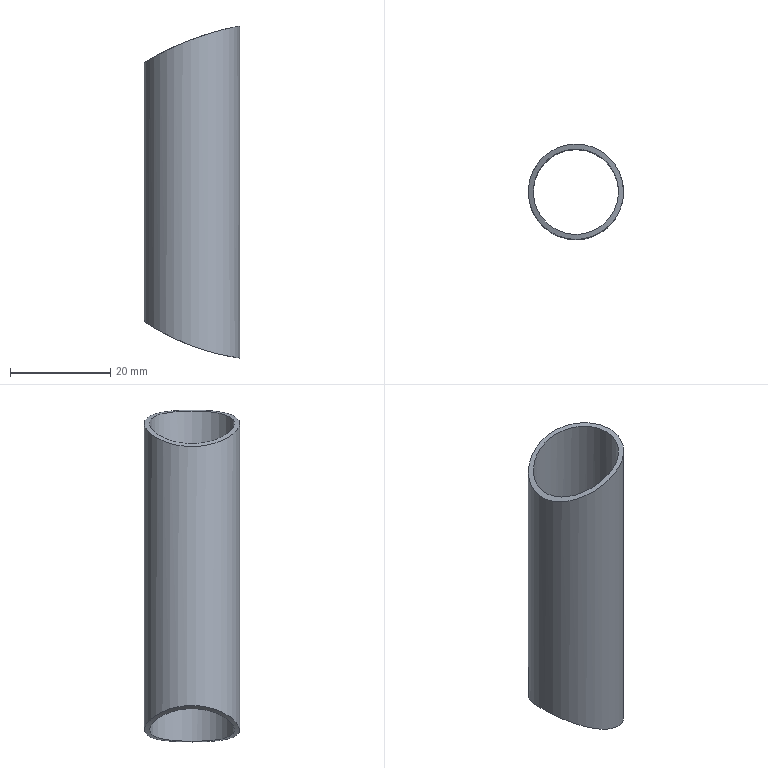Part | STEP file | 1-57.3 | 1 solid | 4 faces | box 19.001 x 19.001 x 66.2 mm | volume 3399 mm3 | cylinder 4 | commonest cylinder face diameters 17 x1 19 x1 92 x1 116.4 x1
STEP:
#1=CARTESIAN_POINT('',(0.,0.,0.));
#2=DIRECTION('',(0.,0.,1.));
#3=DIRECTION('',(1.,0.,0.));
#4=AXIS2_PLACEMENT_3D('',#1,#2,#3);
#5=CARTESIAN_POINT('',(9.5,0.00000001,33.1));
#6=VERTEX_POINT('',#5);
#7=CARTESIAN_POINT('',(9.5,0.000000021,33.1));
#8=CARTESIAN_POINT('',(9.5,1.036,33.1));
#9=CARTESIAN_POINT('',(8.992,4.143,33.002));
#10=CARTESIAN_POINT('',(7.036,6.692,32.594));
#11=CARTESIAN_POINT('',(3.324,9.242,31.592));
#12=CARTESIAN_POINT('',(0.8782,9.747,30.79));
#13=CARTESIAN_POINT('',(-3.995,8.997,28.801));
#14=CARTESIAN_POINT('',(-6.328,7.57,27.609));
#15=CARTESIAN_POINT('',(-9.203,3.377,26.002));
#16=CARTESIAN_POINT('',(-9.792,0.8976,25.625));
#17=CARTESIAN_POINT('',(-8.755,-5.155,26.247));
#18=CARTESIAN_POINT('',(-6.252,-7.864,27.729));
#19=CARTESIAN_POINT('',(-0.9257,-9.75,30.107));
#20=CARTESIAN_POINT('',(1.596,-9.694,31.037));
#21=CARTESIAN_POINT('',(6.765,-7.38,32.582));
#22=CARTESIAN_POINT('',(8.887,-4.697,32.98));
#23=CARTESIAN_POINT('',(9.438,-1.131,33.088));
#24=CARTESIAN_POINT('',(9.488,-0.6473,33.098));
#25=CARTESIAN_POINT('',(9.5,-0.1618,33.1));
#26=CARTESIAN_POINT('',(9.5,0.,33.1));
#27=B_SPLINE_CURVE_WITH_KNOTS('',3,(#7,#8,#9,#10,#11,#12,#13,#14,#15,#16,#17,#18,#19,#20,#21,#22,#23,#24,#25,#26),.UNSPECIFIED.,.F.,.F.,(4,1,2,2,2,2,2,2,2,1,4),(0.000000002,0.3333,1.,1.826,2.733,3.556,4.725,5.575,6.649,6.755,6.808),.UNSPECIFIED.);
#28=CARTESIAN_POINT('',(0.,0.,33.1));
#29=DIRECTION('',(0.,0.,-1.));
#30=DIRECTION('',(1.,0.,0.));
#31=AXIS2_PLACEMENT_3D('',#28,#29,#30);
#32=CYLINDRICAL_SURFACE('',#31,9.5);
#33=CARTESIAN_POINT('',(6.283,0.));
#34=CARTESIAN_POINT('',(6.233,0.00002118));
#35=CARTESIAN_POINT('',(6.131,0.0141));
#36=CARTESIAN_POINT('',(5.98,0.07863));
#37=CARTESIAN_POINT('',(5.83,0.1873));
#38=CARTESIAN_POINT('',(5.68,0.3429));
#39=CARTESIAN_POINT('',(5.531,0.5482));
#40=CARTESIAN_POINT('',(5.382,0.806));
#41=CARTESIAN_POINT('',(5.235,1.12));
#42=CARTESIAN_POINT('',(5.091,1.484));
#43=CARTESIAN_POINT('',(4.95,1.894));
#44=CARTESIAN_POINT('',(4.81,2.346));
#45=CARTESIAN_POINT('',(4.671,2.835));
#46=CARTESIAN_POINT('',(4.532,3.36));
#47=CARTESIAN_POINT('',(4.394,3.91));
#48=CARTESIAN_POINT('',(4.255,4.468));
#49=CARTESIAN_POINT('',(4.117,5.02));
#50=CARTESIAN_POINT('',(3.978,5.55));
#51=CARTESIAN_POINT('',(3.838,6.043));
#52=CARTESIAN_POINT('',(3.694,6.488));
#53=CARTESIAN_POINT('',(3.551,6.848));
#54=CARTESIAN_POINT('',(3.408,7.113));
#55=CARTESIAN_POINT('',(3.264,7.273));
#56=CARTESIAN_POINT('',(3.119,7.318));
#57=CARTESIAN_POINT('',(2.97,7.237));
#58=CARTESIAN_POINT('',(2.821,7.03));
#59=CARTESIAN_POINT('',(2.677,6.725));
#60=CARTESIAN_POINT('',(2.536,6.336));
#61=CARTESIAN_POINT('',(2.397,5.881));
#62=CARTESIAN_POINT('',(2.259,5.377));
#63=CARTESIAN_POINT('',(2.121,4.84));
#64=CARTESIAN_POINT('',(1.984,4.289));
#65=CARTESIAN_POINT('',(1.848,3.74));
#66=CARTESIAN_POINT('',(1.711,3.21));
#67=CARTESIAN_POINT('',(1.574,2.703));
#68=CARTESIAN_POINT('',(1.437,2.225));
#69=CARTESIAN_POINT('',(1.298,1.784));
#70=CARTESIAN_POINT('',(1.155,1.384));
#71=CARTESIAN_POINT('',(1.012,1.037));
#72=CARTESIAN_POINT('',(0.8697,0.7468));
#73=CARTESIAN_POINT('',(0.7278,0.508));
#74=CARTESIAN_POINT('',(0.5857,0.3183));
#75=CARTESIAN_POINT('',(0.4425,0.1747));
#76=CARTESIAN_POINT('',(0.2978,0.07458));
#77=CARTESIAN_POINT('',(0.1497,0.01389));
#78=CARTESIAN_POINT('',(0.04999,0.0002314));
#79=CARTESIAN_POINT('',(0.,0.));
#80=B_SPLINE_CURVE_WITH_KNOTS('',3,(#33,#34,#35,#36,#37,#38,#39,#40,#41,#42,#43,#44,#45,#46,#47,#48,#49,#50,#51,#52,#53,#54,#55,#56,#57,#58,#59,#60,#61,#62,#63,#64,#65,#66,#67,#68,#69,#70,#71,#72,#73,#74,#75,#76,#77,#78,#79),.UNSPECIFIED.,.F.,.F.,(4,1,1,1,1,1,1,1,1,1,1,1,1,1,1,1,1,1,1,1,1,1,1,1,1,1,1,1,1,1,1,1,1,1,1,1,1,1,1,1,1,1,1,1,4),(0.000000002,0.1547,0.3094,0.4641,0.6189,0.7736,0.9283,1.083,1.238,1.392,1.547,1.702,1.857,2.011,2.166,2.321,2.475,2.63,2.785,2.94,3.094,3.249,3.404,3.558,3.713,3.868,4.023,4.177,4.332,4.487,4.641,4.796,4.951,5.106,5.26,5.415,5.57,5.724,5.879,6.034,6.189,6.343,6.498,6.653,6.808),.QUASI_UNIFORM_KNOTS.);
#81=(GEOMETRIC_REPRESENTATION_CONTEXT(2)PARAMETRIC_REPRESENTATION_CONTEXT()REPRESENTATION_CONTEXT('',''));
#82=DEFINITIONAL_REPRESENTATION('',(#80),#81);
#83=PCURVE('',#32,#82);
#84=CARTESIAN_POINT('',(20.552,-33.1,-24.041));
#85=DIRECTION('',(0.,1.,0.));
#86=DIRECTION('',(-0.5164,0.,0.8564));
#87=AXIS2_PLACEMENT_3D('',#84,#85,#86);
#88=CYLINDRICAL_SURFACE('',#87,58.2);
#89=CARTESIAN_POINT('',(0.3515,33.1));
#90=CARTESIAN_POINT('',(0.3515,33.581));
#91=CARTESIAN_POINT('',(0.3503,34.542));
#92=CARTESIAN_POINT('',(0.3446,35.947));
#93=CARTESIAN_POINT('',(0.3353,37.277));
#94=CARTESIAN_POINT('',(0.3226,38.507));
#95=CARTESIAN_POINT('',(0.3068,39.613));
#96=CARTESIAN_POINT('',(0.2885,40.573));
#97=CARTESIAN_POINT('',(0.2678,41.361));
#98=CARTESIAN_POINT('',(0.2458,41.956));
#99=CARTESIAN_POINT('',(0.2226,42.364));
#100=CARTESIAN_POINT('',(0.1987,42.586));
#101=CARTESIAN_POINT('',(0.1745,42.623));
#102=CARTESIAN_POINT('',(0.1501,42.476));
#103=CARTESIAN_POINT('',(0.1262,42.15));
#104=CARTESIAN_POINT('',(0.1032,41.652));
#105=CARTESIAN_POINT('',(0.08148,40.991));
#106=CARTESIAN_POINT('',(0.06137,40.174));
#107=CARTESIAN_POINT('',(0.04331,39.211));
#108=CARTESIAN_POINT('',(0.02759,38.103));
#109=CARTESIAN_POINT('',(0.01512,36.896));
#110=CARTESIAN_POINT('',(0.006102,35.612));
#111=CARTESIAN_POINT('',(0.0007772,34.268));
#112=CARTESIAN_POINT('',(-0.0006513,32.886));
#113=CARTESIAN_POINT('',(0.002114,31.468));
#114=CARTESIAN_POINT('',(0.009037,30.094));
#115=CARTESIAN_POINT('',(0.01946,28.831));
#116=CARTESIAN_POINT('',(0.03303,27.675));
#117=CARTESIAN_POINT('',(0.04932,26.641));
#118=CARTESIAN_POINT('',(0.06791,25.739));
#119=CARTESIAN_POINT('',(0.08839,24.98));
#120=CARTESIAN_POINT('',(0.1104,24.374));
#121=CARTESIAN_POINT('',(0.1334,23.933));
#122=CARTESIAN_POINT('',(0.1571,23.664));
#123=CARTESIAN_POINT('',(0.181,23.569));
#124=CARTESIAN_POINT('',(0.205,23.654));
#125=CARTESIAN_POINT('',(0.2285,23.922));
#126=CARTESIAN_POINT('',(0.2515,24.378));
#127=CARTESIAN_POINT('',(0.2731,25.019));
#128=CARTESIAN_POINT('',(0.2925,25.817));
#129=CARTESIAN_POINT('',(0.3097,26.759));
#130=CARTESIAN_POINT('',(0.3242,27.831));
#131=CARTESIAN_POINT('',(0.336,29.018));
#132=CARTESIAN_POINT('',(0.3448,30.302));
#133=CARTESIAN_POINT('',(0.3503,31.678));
#134=CARTESIAN_POINT('',(0.3515,32.625));
#135=CARTESIAN_POINT('',(0.3515,33.1));
#136=B_SPLINE_CURVE_WITH_KNOTS('',3,(#89,#90,#91,#92,#93,#94,#95,#96,#97,#98,#99,#100,#101,#102,#103,#104,#105,#106,#107,#108,#109,#110,#111,#112,#113,#114,#115,#116,#117,#118,#119,#120,#121,#122,#123,#124,#125,#126,#127,#128,#129,#130,#131,#132,#133,#134,#135),.UNSPECIFIED.,.F.,.F.,(4,1,1,1,1,1,1,1,1,1,1,1,1,1,1,1,1,1,1,1,1,1,1,1,1,1,1,1,1,1,1,1,1,1,1,1,1,1,1,1,1,1,1,1,4),(0.000000002,0.1547,0.3094,0.4641,0.6189,0.7736,0.9283,1.083,1.238,1.392,1.547,1.702,1.857,2.011,2.166,2.321,2.475,2.63,2.785,2.94,3.094,3.249,3.404,3.558,3.713,3.868,4.023,4.177,4.332,4.487,4.641,4.796,4.951,5.106,5.26,5.415,5.57,5.724,5.879,6.034,6.189,6.343,6.498,6.653,6.808),.QUASI_UNIFORM_KNOTS.);
#137=(GEOMETRIC_REPRESENTATION_CONTEXT(2)PARAMETRIC_REPRESENTATION_CONTEXT()REPRESENTATION_CONTEXT('',''));
#138=DEFINITIONAL_REPRESENTATION('',(#136),#137);
#139=PCURVE('',#88,#138);
#140=SURFACE_CURVE('',#27,(#83,#139),.PCURVE_S1.);
#141=EDGE_CURVE('',#6,#6,#140,.T.);
#142=ORIENTED_EDGE('',*,*,#141,.F.);
#143=CARTESIAN_POINT('',(9.5,0.,-33.1));
#144=VERTEX_POINT('',#143);
#145=CARTESIAN_POINT('',(9.5,0.,33.1));
#146=DIRECTION('',(0.,0.,-1.));
#147=VECTOR('',#146,1.);
#148=LINE('',#145,#147);
#149=CARTESIAN_POINT('',(6.283,0.));
#150=DIRECTION('',(0.,1.));
#151=VECTOR('',#150,1.);
#152=LINE('',#149,#151);
#153=(GEOMETRIC_REPRESENTATION_CONTEXT(2)PARAMETRIC_REPRESENTATION_CONTEXT()REPRESENTATION_CONTEXT('',''));
#154=DEFINITIONAL_REPRESENTATION('',(#152),#153);
#155=PCURVE('',#32,#154);
#156=CARTESIAN_POINT('',(0.,0.));
#157=DIRECTION('',(0.,1.));
#158=VECTOR('',#157,1.);
#159=LINE('',#156,#158);
#160=(GEOMETRIC_REPRESENTATION_CONTEXT(2)PARAMETRIC_REPRESENTATION_CONTEXT()REPRESENTATION_CONTEXT('',''));
#161=DEFINITIONAL_REPRESENTATION('',(#159),#160);
#162=PCURVE('',#32,#161);
#163=SEAM_CURVE('',#148,(#155,#162),.PCURVE_S1.);
#164=EDGE_CURVE('',#6,#144,#163,.T.);
#165=ORIENTED_EDGE('',*,*,#164,.T.);
#166=CARTESIAN_POINT('',(9.5,0.,-33.1));
#167=CARTESIAN_POINT('',(9.5,-1.046,-33.1));
#168=CARTESIAN_POINT('',(8.981,-4.186,-33.025));
#169=CARTESIAN_POINT('',(6.985,-6.756,-32.698));
#170=CARTESIAN_POINT('',(3.23,-9.271,-31.791));
#171=CARTESIAN_POINT('',(0.8082,-9.745,-31.033));
#172=CARTESIAN_POINT('',(-3.78,-9.021,-29.136));
#173=CARTESIAN_POINT('',(-5.885,-7.822,-28.024));
#174=CARTESIAN_POINT('',(-8.869,-4.15,-26.254));
#175=CARTESIAN_POINT('',(-9.68,-1.751,-25.68));
#176=CARTESIAN_POINT('',(-9.166,4.378,-26.023));
#177=CARTESIAN_POINT('',(-6.919,7.261,-27.539));
#178=CARTESIAN_POINT('',(-2.119,9.491,-29.869));
#179=CARTESIAN_POINT('',(0.04298,9.745,-30.742));
#180=CARTESIAN_POINT('',(5.805,8.401,-32.573));
#181=CARTESIAN_POINT('',(8.729,5.438,-32.986));
#182=CARTESIAN_POINT('',(9.429,1.209,-33.09));
#183=CARTESIAN_POINT('',(9.486,0.6924,-33.098));
#184=CARTESIAN_POINT('',(9.5,0.1731,-33.1));
#185=CARTESIAN_POINT('',(9.5,0.,-33.1));
#186=B_SPLINE_CURVE_WITH_KNOTS('',3,(#166,#167,#168,#169,#170,#171,#172,#173,#174,#175,#176,#177,#178,#179,#180,#181,#182,#183,#184,#185),.UNSPECIFIED.,.T.,.F.,(1,3,1,2,2,2,2,2,2,2,1,3,1),(-0.05615,0.,0.3333,1.,1.807,2.617,3.432,4.581,5.323,6.601,6.713,6.769,7.103),.UNSPECIFIED.);
#187=CARTESIAN_POINT('',(0.,66.2));
#188=CARTESIAN_POINT('',(0.05086,66.2));
#189=CARTESIAN_POINT('',(0.1525,66.189));
#190=CARTESIAN_POINT('',(0.3046,66.14));
#191=CARTESIAN_POINT('',(0.4557,66.055));
#192=CARTESIAN_POINT('',(0.6064,65.929));
#193=CARTESIAN_POINT('',(0.7566,65.757));
#194=CARTESIAN_POINT('',(0.9062,65.532));
#195=CARTESIAN_POINT('',(1.055,65.248));
#196=CARTESIAN_POINT('',(1.2,64.908));
#197=CARTESIAN_POINT('',(1.343,64.516));
#198=CARTESIAN_POINT('',(1.483,64.074));
#199=CARTESIAN_POINT('',(1.623,63.586));
#200=CARTESIAN_POINT('',(1.763,63.053));
#201=CARTESIAN_POINT('',(1.902,62.487));
#202=CARTESIAN_POINT('',(2.04,61.907));
#203=CARTESIAN_POINT('',(2.178,61.328));
#204=CARTESIAN_POINT('',(2.317,60.767));
#205=CARTESIAN_POINT('',(2.457,60.237));
#206=CARTESIAN_POINT('',(2.599,59.766));
#207=CARTESIAN_POINT('',(2.741,59.379));
#208=CARTESIAN_POINT('',(2.884,59.092));
#209=CARTESIAN_POINT('',(3.029,58.92));
#210=CARTESIAN_POINT('',(3.177,58.879));
#211=CARTESIAN_POINT('',(3.33,58.989));
#212=CARTESIAN_POINT('',(3.475,59.226));
#213=CARTESIAN_POINT('',(3.618,59.57));
#214=CARTESIAN_POINT('',(3.758,60.001));
#215=CARTESIAN_POINT('',(3.897,60.498));
#216=CARTESIAN_POINT('',(4.035,61.041));
#217=CARTESIAN_POINT('',(4.172,61.609));
#218=CARTESIAN_POINT('',(4.308,62.182));
#219=CARTESIAN_POINT('',(4.444,62.742));
#220=CARTESIAN_POINT('',(4.58,63.282));
#221=CARTESIAN_POINT('',(4.717,63.791));
#222=CARTESIAN_POINT('',(4.856,64.262));
#223=CARTESIAN_POINT('',(4.999,64.688));
#224=CARTESIAN_POINT('',(5.14,65.049));
#225=CARTESIAN_POINT('',(5.279,65.351));
#226=CARTESIAN_POINT('',(5.419,65.6));
#227=CARTESIAN_POINT('',(5.559,65.799));
#228=CARTESIAN_POINT('',(5.699,65.953));
#229=CARTESIAN_POINT('',(5.841,66.067));
#230=CARTESIAN_POINT('',(5.985,66.144));
#231=CARTESIAN_POINT('',(6.133,66.19));
#232=CARTESIAN_POINT('',(6.233,66.2));
#233=CARTESIAN_POINT('',(6.283,66.2));
#234=B_SPLINE_CURVE_WITH_KNOTS('',3,(#187,#188,#189,#190,#191,#192,#193,#194,#195,#196,#197,#198,#199,#200,#201,#202,#203,#204,#205,#206,#207,#208,#209,#210,#211,#212,#213,#214,#215,#216,#217,#218,#219,#220,#221,#222,#223,#224,#225,#226,#227,#228,#229,#230,#231,#232,#233),.UNSPECIFIED.,.F.,.F.,(4,1,1,1,1,1,1,1,1,1,1,1,1,1,1,1,1,1,1,1,1,1,1,1,1,1,1,1,1,1,1,1,1,1,1,1,1,1,1,1,1,1,1,1,4),(0.,0.1538,0.3077,0.4615,0.6154,0.7692,0.9231,1.077,1.231,1.385,1.538,1.692,1.846,2.,2.154,2.308,2.462,2.615,2.769,2.923,3.077,3.231,3.385,3.538,3.692,3.846,4.,4.154,4.308,4.462,4.615,4.769,4.923,5.077,5.231,5.385,5.538,5.692,5.846,6.,6.154,6.308,6.461,6.615,6.769),.QUASI_UNIFORM_KNOTS.);
#235=(GEOMETRIC_REPRESENTATION_CONTEXT(2)PARAMETRIC_REPRESENTATION_CONTEXT()REPRESENTATION_CONTEXT('',''));
#236=DEFINITIONAL_REPRESENTATION('',(#234),#235);
#237=PCURVE('',#32,#236);
#238=CARTESIAN_POINT('',(16.089,-33.1,12.426));
#239=DIRECTION('',(0.,1.,0.));
#240=DIRECTION('',(-0.1432,0.,-0.9897));
#241=AXIS2_PLACEMENT_3D('',#238,#239,#240);
#242=CYLINDRICAL_SURFACE('',#241,46.);
#243=CARTESIAN_POINT('',(0.,33.1));
#244=CARTESIAN_POINT('',(-0.000003529,32.617));
#245=CARTESIAN_POINT('',(0.00162,31.651));
#246=CARTESIAN_POINT('',(0.00879,30.239));
#247=CARTESIAN_POINT('',(0.02063,28.903));
#248=CARTESIAN_POINT('',(0.03674,27.668));
#249=CARTESIAN_POINT('',(0.05668,26.557));
#250=CARTESIAN_POINT('',(0.08002,25.594));
#251=CARTESIAN_POINT('',(0.1064,24.804));
#252=CARTESIAN_POINT('',(0.1345,24.213));
#253=CARTESIAN_POINT('',(0.164,23.814));
#254=CARTESIAN_POINT('',(0.1943,23.604));
#255=CARTESIAN_POINT('',(0.2252,23.582));
#256=CARTESIAN_POINT('',(0.2561,23.745));
#257=CARTESIAN_POINT('',(0.2864,24.087));
#258=CARTESIAN_POINT('',(0.3156,24.599));
#259=CARTESIAN_POINT('',(0.3433,25.274));
#260=CARTESIAN_POINT('',(0.3688,26.101));
#261=CARTESIAN_POINT('',(0.3918,27.076));
#262=CARTESIAN_POINT('',(0.4116,28.179));
#263=CARTESIAN_POINT('',(0.4273,29.382));
#264=CARTESIAN_POINT('',(0.4388,30.671));
#265=CARTESIAN_POINT('',(0.4455,32.029));
#266=CARTESIAN_POINT('',(0.447,33.442));
#267=CARTESIAN_POINT('',(0.4427,34.884));
#268=CARTESIAN_POINT('',(0.4334,36.223));
#269=CARTESIAN_POINT('',(0.4195,37.472));
#270=CARTESIAN_POINT('',(0.4017,38.612));
#271=CARTESIAN_POINT('',(0.3805,39.633));
#272=CARTESIAN_POINT('',(0.3565,40.522));
#273=CARTESIAN_POINT('',(0.3302,41.269));
#274=CARTESIAN_POINT('',(0.3022,41.859));
#275=CARTESIAN_POINT('',(0.273,42.287));
#276=CARTESIAN_POINT('',(0.2429,42.547));
#277=CARTESIAN_POINT('',(0.2125,42.631));
#278=CARTESIAN_POINT('',(0.182,42.533));
#279=CARTESIAN_POINT('',(0.1517,42.244));
#280=CARTESIAN_POINT('',(0.1233,41.774));
#281=CARTESIAN_POINT('',(0.09705,41.139));
#282=CARTESIAN_POINT('',(0.07321,40.35));
#283=CARTESIAN_POINT('',(0.05211,39.419));
#284=CARTESIAN_POINT('',(0.03407,38.359));
#285=CARTESIAN_POINT('',(0.01942,37.183));
#286=CARTESIAN_POINT('',(0.008493,35.904));
#287=CARTESIAN_POINT('',(0.001587,34.525));
#288=CARTESIAN_POINT('',(-0.00001821,33.576));
#289=CARTESIAN_POINT('',(0.,33.1));
#290=B_SPLINE_CURVE_WITH_KNOTS('',3,(#243,#244,#245,#246,#247,#248,#249,#250,#251,#252,#253,#254,#255,#256,#257,#258,#259,#260,#261,#262,#263,#264,#265,#266,#267,#268,#269,#270,#271,#272,#273,#274,#275,#276,#277,#278,#279,#280,#281,#282,#283,#284,#285,#286,#287,#288,#289),.UNSPECIFIED.,.T.,.F.,(4,1,1,1,1,1,1,1,1,1,1,1,1,1,1,1,1,1,1,1,1,1,1,1,1,1,1,1,1,1,1,1,1,1,1,1,1,1,1,1,1,1,1,1,4),(0.,0.1538,0.3077,0.4615,0.6154,0.7692,0.9231,1.077,1.231,1.385,1.538,1.692,1.846,2.,2.154,2.308,2.462,2.615,2.769,2.923,3.077,3.231,3.385,3.538,3.692,3.846,4.,4.154,4.308,4.462,4.615,4.769,4.923,5.077,5.231,5.385,5.538,5.692,5.846,6.,6.154,6.308,6.461,6.615,6.769),.QUASI_UNIFORM_KNOTS.);
#291=(GEOMETRIC_REPRESENTATION_CONTEXT(2)PARAMETRIC_REPRESENTATION_CONTEXT()REPRESENTATION_CONTEXT('',''));
#292=DEFINITIONAL_REPRESENTATION('',(#290),#291);
#293=PCURVE('',#242,#292);
#294=SURFACE_CURVE('',#186,(#237,#293),.PCURVE_S1.);
#295=EDGE_CURVE('',#144,#144,#294,.T.);
#296=ORIENTED_EDGE('',*,*,#295,.F.);
#297=ORIENTED_EDGE('',*,*,#164,.F.);
#298=EDGE_LOOP('',(#142,#165,#296,#297));
#299=FACE_BOUND('',#298,.T.);
#300=ADVANCED_FACE('',(#299),#32,.T.);
#301=CARTESIAN_POINT('',(8.5,0.,32.897));
#302=VERTEX_POINT('',#301);
#303=CARTESIAN_POINT('',(8.5,0.,-32.944));
#304=VERTEX_POINT('',#303);
#305=CARTESIAN_POINT('',(8.5,0.,32.897));
#306=DIRECTION('',(0.,0.,-1.));
#307=VECTOR('',#306,1.);
#308=LINE('',#305,#307);
#309=CARTESIAN_POINT('',(0.,0.,33.1));
#310=DIRECTION('',(0.,0.,-1.));
#311=DIRECTION('',(1.,0.,0.));
#312=AXIS2_PLACEMENT_3D('',#309,#310,#311);
#313=CYLINDRICAL_SURFACE('',#312,8.5);
#314=CARTESIAN_POINT('',(0.,0.2025));
#315=DIRECTION('',(0.,1.));
#316=VECTOR('',#315,1.);
#317=LINE('',#314,#316);
#318=(GEOMETRIC_REPRESENTATION_CONTEXT(2)PARAMETRIC_REPRESENTATION_CONTEXT()REPRESENTATION_CONTEXT('',''));
#319=DEFINITIONAL_REPRESENTATION('',(#317),#318);
#320=PCURVE('',#313,#319);
#321=CARTESIAN_POINT('',(6.283,0.2025));
#322=DIRECTION('',(0.,1.));
#323=VECTOR('',#322,1.);
#324=LINE('',#321,#323);
#325=(GEOMETRIC_REPRESENTATION_CONTEXT(2)PARAMETRIC_REPRESENTATION_CONTEXT()REPRESENTATION_CONTEXT('',''));
#326=DEFINITIONAL_REPRESENTATION('',(#324),#325);
#327=PCURVE('',#313,#326);
#328=SEAM_CURVE('',#308,(#320,#327),.PCURVE_S1.);
#329=EDGE_CURVE('',#302,#304,#328,.T.);
#330=ORIENTED_EDGE('',*,*,#329,.F.);
#331=CARTESIAN_POINT('',(8.5,0.,32.897));
#332=CARTESIAN_POINT('',(8.5,-0.8945,32.897));
#333=CARTESIAN_POINT('',(8.076,-3.578,32.808));
#334=CARTESIAN_POINT('',(6.442,-5.811,32.441));
#335=CARTESIAN_POINT('',(3.108,-8.269,31.52));
#336=CARTESIAN_POINT('',(0.7372,-8.766,30.735));
#337=CARTESIAN_POINT('',(-3.877,-7.942,28.846));
#338=CARTESIAN_POINT('',(-6.035,-6.499,27.752));
#339=CARTESIAN_POINT('',(-8.364,-2.552,26.482));
#340=CARTESIAN_POINT('',(-8.75,-0.4462,26.247));
#341=CARTESIAN_POINT('',(-7.729,4.75,26.831));
#342=CARTESIAN_POINT('',(-5.491,7.104,28.093));
#343=CARTESIAN_POINT('',(-0.6997,8.745,30.187));
#344=CARTESIAN_POINT('',(1.596,8.652,31.027));
#345=CARTESIAN_POINT('',(6.352,6.392,32.471));
#346=CARTESIAN_POINT('',(8.248,3.732,32.844));
#347=CARTESIAN_POINT('',(8.487,0.4856,32.895));
#348=CARTESIAN_POINT('',(8.497,0.2775,32.897));
#349=CARTESIAN_POINT('',(8.5,0.06938,32.897));
#350=CARTESIAN_POINT('',(8.5,0.,32.897));
#351=B_SPLINE_CURVE_WITH_KNOTS('',3,(#331,#332,#333,#334,#335,#336,#337,#338,#339,#340,#341,#342,#343,#344,#345,#346,#347,#348,#349,#350),.UNSPECIFIED.,.T.,.F.,(1,3,1,2,2,2,2,2,2,2,1,3,1),(-0.02621,0.,0.3333,1.,1.922,2.908,3.707,4.9,5.794,6.972,7.024,7.05,7.384),.UNSPECIFIED.);
#352=CARTESIAN_POINT('',(0.,0.2025));
#353=CARTESIAN_POINT('',(0.05061,0.2025));
#354=CARTESIAN_POINT('',(0.1518,0.2163));
#355=CARTESIAN_POINT('',(0.303,0.2791));
#356=CARTESIAN_POINT('',(0.4533,0.3844));
#357=CARTESIAN_POINT('',(0.6031,0.5338));
#358=CARTESIAN_POINT('',(0.7521,0.7289));
#359=CARTESIAN_POINT('',(0.9003,0.9715));
#360=CARTESIAN_POINT('',(1.047,1.263));
#361=CARTESIAN_POINT('',(1.19,1.596));
#362=CARTESIAN_POINT('',(1.331,1.967));
#363=CARTESIAN_POINT('',(1.47,2.374));
#364=CARTESIAN_POINT('',(1.609,2.811));
#365=CARTESIAN_POINT('',(1.748,3.276));
#366=CARTESIAN_POINT('',(1.887,3.762));
#367=CARTESIAN_POINT('',(2.025,4.252));
#368=CARTESIAN_POINT('',(2.163,4.736));
#369=CARTESIAN_POINT('',(2.303,5.198));
#370=CARTESIAN_POINT('',(2.444,5.627));
#371=CARTESIAN_POINT('',(2.587,6.009));
#372=CARTESIAN_POINT('',(2.732,6.326));
#373=CARTESIAN_POINT('',(2.876,6.553));
#374=CARTESIAN_POINT('',(3.021,6.689));
#375=CARTESIAN_POINT('',(3.167,6.725));
#376=CARTESIAN_POINT('',(3.315,6.655));
#377=CARTESIAN_POINT('',(3.465,6.476));
#378=CARTESIAN_POINT('',(3.609,6.212));
#379=CARTESIAN_POINT('',(3.75,5.875));
#380=CARTESIAN_POINT('',(3.89,5.481));
#381=CARTESIAN_POINT('',(4.028,5.042));
#382=CARTESIAN_POINT('',(4.166,4.574));
#383=CARTESIAN_POINT('',(4.303,4.09));
#384=CARTESIAN_POINT('',(4.441,3.606));
#385=CARTESIAN_POINT('',(4.577,3.135));
#386=CARTESIAN_POINT('',(4.714,2.683));
#387=CARTESIAN_POINT('',(4.852,2.256));
#388=CARTESIAN_POINT('',(4.991,1.859));
#389=CARTESIAN_POINT('',(5.133,1.496));
#390=CARTESIAN_POINT('',(5.277,1.177));
#391=CARTESIAN_POINT('',(5.419,0.9077));
#392=CARTESIAN_POINT('',(5.56,0.6842));
#393=CARTESIAN_POINT('',(5.702,0.5052));
#394=CARTESIAN_POINT('',(5.844,0.3687));
#395=CARTESIAN_POINT('',(5.987,0.273));
#396=CARTESIAN_POINT('',(6.134,0.2159));
#397=CARTESIAN_POINT('',(6.233,0.203));
#398=CARTESIAN_POINT('',(6.283,0.2025));
#399=B_SPLINE_CURVE_WITH_KNOTS('',3,(#352,#353,#354,#355,#356,#357,#358,#359,#360,#361,#362,#363,#364,#365,#366,#367,#368,#369,#370,#371,#372,#373,#374,#375,#376,#377,#378,#379,#380,#381,#382,#383,#384,#385,#386,#387,#388,#389,#390,#391,#392,#393,#394,#395,#396,#397,#398),.UNSPECIFIED.,.F.,.F.,(4,1,1,1,1,1,1,1,1,1,1,1,1,1,1,1,1,1,1,1,1,1,1,1,1,1,1,1,1,1,1,1,1,1,1,1,1,1,1,1,1,1,1,1,4),(0.,0.1602,0.3205,0.4807,0.6409,0.8012,0.9614,1.122,1.282,1.442,1.602,1.763,1.923,2.083,2.243,2.404,2.564,2.724,2.884,3.044,3.205,3.365,3.525,3.685,3.846,4.006,4.166,4.326,4.487,4.647,4.807,4.967,5.128,5.288,5.448,5.608,5.768,5.929,6.089,6.249,6.409,6.57,6.73,6.89,7.05),.QUASI_UNIFORM_KNOTS.);
#400=(GEOMETRIC_REPRESENTATION_CONTEXT(2)PARAMETRIC_REPRESENTATION_CONTEXT()REPRESENTATION_CONTEXT('',''));
#401=DEFINITIONAL_REPRESENTATION('',(#399),#400);
#402=PCURVE('',#313,#401);
#403=CARTESIAN_POINT('',(0.334,33.1));
#404=CARTESIAN_POINT('',(0.334,32.67));
#405=CARTESIAN_POINT('',(0.3329,31.81));
#406=CARTESIAN_POINT('',(0.3278,30.553));
#407=CARTESIAN_POINT('',(0.3194,29.364));
#408=CARTESIAN_POINT('',(0.308,28.263));
#409=CARTESIAN_POINT('',(0.2939,27.274));
#410=CARTESIAN_POINT('',(0.2775,26.415));
#411=CARTESIAN_POINT('',(0.259,25.714));
#412=CARTESIAN_POINT('',(0.2393,25.182));
#413=CARTESIAN_POINT('',(0.2187,24.816));
#414=CARTESIAN_POINT('',(0.1974,24.615));
#415=CARTESIAN_POINT('',(0.1757,24.579));
#416=CARTESIAN_POINT('',(0.154,24.706));
#417=CARTESIAN_POINT('',(0.1326,24.995));
#418=CARTESIAN_POINT('',(0.112,25.438));
#419=CARTESIAN_POINT('',(0.09259,26.027));
#420=CARTESIAN_POINT('',(0.07463,26.757));
#421=CARTESIAN_POINT('',(0.05852,27.618));
#422=CARTESIAN_POINT('',(0.04456,28.607));
#423=CARTESIAN_POINT('',(0.03329,29.705));
#424=CARTESIAN_POINT('',(0.02528,30.863));
#425=CARTESIAN_POINT('',(0.02058,32.073));
#426=CARTESIAN_POINT('',(0.01939,33.313));
#427=CARTESIAN_POINT('',(0.02186,34.573));
#428=CARTESIAN_POINT('',(0.02806,35.809));
#429=CARTESIAN_POINT('',(0.03737,36.94));
#430=CARTESIAN_POINT('',(0.04948,37.976));
#431=CARTESIAN_POINT('',(0.06402,38.9));
#432=CARTESIAN_POINT('',(0.08063,39.707));
#433=CARTESIAN_POINT('',(0.09895,40.384));
#434=CARTESIAN_POINT('',(0.1186,40.923));
#435=CARTESIAN_POINT('',(0.1393,41.314));
#436=CARTESIAN_POINT('',(0.1605,41.549));
#437=CARTESIAN_POINT('',(0.182,41.627));
#438=CARTESIAN_POINT('',(0.2034,41.545));
#439=CARTESIAN_POINT('',(0.2245,41.299));
#440=CARTESIAN_POINT('',(0.2449,40.886));
#441=CARTESIAN_POINT('',(0.2643,40.306));
#442=CARTESIAN_POINT('',(0.2816,39.588));
#443=CARTESIAN_POINT('',(0.2969,38.743));
#444=CARTESIAN_POINT('',(0.3098,37.785));
#445=CARTESIAN_POINT('',(0.3203,36.728));
#446=CARTESIAN_POINT('',(0.328,35.586));
#447=CARTESIAN_POINT('',(0.3329,34.372));
#448=CARTESIAN_POINT('',(0.334,33.528));
#449=CARTESIAN_POINT('',(0.334,33.1));
#450=B_SPLINE_CURVE_WITH_KNOTS('',3,(#403,#404,#405,#406,#407,#408,#409,#410,#411,#412,#413,#414,#415,#416,#417,#418,#419,#420,#421,#422,#423,#424,#425,#426,#427,#428,#429,#430,#431,#432,#433,#434,#435,#436,#437,#438,#439,#440,#441,#442,#443,#444,#445,#446,#447,#448,#449),.UNSPECIFIED.,.T.,.F.,(4,1,1,1,1,1,1,1,1,1,1,1,1,1,1,1,1,1,1,1,1,1,1,1,1,1,1,1,1,1,1,1,1,1,1,1,1,1,1,1,1,1,1,1,4),(0.,0.1602,0.3205,0.4807,0.6409,0.8012,0.9614,1.122,1.282,1.442,1.602,1.763,1.923,2.083,2.243,2.404,2.564,2.724,2.884,3.044,3.205,3.365,3.525,3.685,3.846,4.006,4.166,4.326,4.487,4.647,4.807,4.967,5.128,5.288,5.448,5.608,5.768,5.929,6.089,6.249,6.409,6.57,6.73,6.89,7.05),.QUASI_UNIFORM_KNOTS.);
#451=(GEOMETRIC_REPRESENTATION_CONTEXT(2)PARAMETRIC_REPRESENTATION_CONTEXT()REPRESENTATION_CONTEXT('',''));
#452=DEFINITIONAL_REPRESENTATION('',(#450),#451);
#453=PCURVE('',#88,#452);
#454=SURFACE_CURVE('',#351,(#402,#453),.PCURVE_S1.);
#455=EDGE_CURVE('',#302,#302,#454,.T.);
#456=ORIENTED_EDGE('',*,*,#455,.T.);
#457=ORIENTED_EDGE('',*,*,#329,.T.);
#458=CARTESIAN_POINT('',(8.5,0.,-32.944));
#459=CARTESIAN_POINT('',(8.5,0.9992,-32.944));
#460=CARTESIAN_POINT('',(7.971,3.997,-32.856));
#461=CARTESIAN_POINT('',(5.952,6.37,-32.477));
#462=CARTESIAN_POINT('',(2.337,8.475,-31.517));
#463=CARTESIAN_POINT('',(0.1034,8.76,-30.766));
#464=CARTESIAN_POINT('',(-4.075,7.77,-28.983));
#465=CARTESIAN_POINT('',(-5.968,6.459,-27.966));
#466=CARTESIAN_POINT('',(-8.272,2.829,-26.615));
#467=CARTESIAN_POINT('',(-8.735,0.7385,-26.304));
#468=CARTESIAN_POINT('',(-7.883,-4.455,-26.839));
#469=CARTESIAN_POINT('',(-5.78,-6.844,-28.147));
#470=CARTESIAN_POINT('',(-1.294,-8.637,-30.213));
#471=CARTESIAN_POINT('',(0.8177,-8.718,-31.015));
#472=CARTESIAN_POINT('',(5.628,-7.037,-32.466));
#473=CARTESIAN_POINT('',(7.8,-4.599,-32.825));
#474=CARTESIAN_POINT('',(8.423,-1.192,-32.931));
#475=CARTESIAN_POINT('',(8.485,-0.6831,-32.941));
#476=CARTESIAN_POINT('',(8.5,-0.1708,-32.944));
#477=CARTESIAN_POINT('',(8.5,0.,-32.944));
#478=B_SPLINE_CURVE_WITH_KNOTS('',3,(#458,#459,#460,#461,#462,#463,#464,#465,#466,#467,#468,#469,#470,#471,#472,#473,#474,#475,#476,#477),.UNSPECIFIED.,.T.,.F.,(1,3,1,2,2,2,2,2,2,2,1,3,1),(-0.05771,0.,0.3333,1.,1.773,2.565,3.283,4.33,5.072,6.127,6.242,6.3,6.633),.UNSPECIFIED.);
#479=CARTESIAN_POINT('',(6.283,66.044));
#480=CARTESIAN_POINT('',(6.233,66.044));
#481=CARTESIAN_POINT('',(6.132,66.033));
#482=CARTESIAN_POINT('',(5.981,65.983));
#483=CARTESIAN_POINT('',(5.831,65.897));
#484=CARTESIAN_POINT('',(5.681,65.774));
#485=CARTESIAN_POINT('',(5.533,65.608));
#486=CARTESIAN_POINT('',(5.385,65.397));
#487=CARTESIAN_POINT('',(5.237,65.136));
#488=CARTESIAN_POINT('',(5.092,64.824));
#489=CARTESIAN_POINT('',(4.95,64.468));
#490=CARTESIAN_POINT('',(4.81,64.071));
#491=CARTESIAN_POINT('',(4.671,63.639));
#492=CARTESIAN_POINT('',(4.532,63.174));
#493=CARTESIAN_POINT('',(4.394,62.681));
#494=CARTESIAN_POINT('',(4.256,62.174));
#495=CARTESIAN_POINT('',(4.117,61.669));
#496=CARTESIAN_POINT('',(3.978,61.18));
#497=CARTESIAN_POINT('',(3.838,60.725));
#498=CARTESIAN_POINT('',(3.695,60.312));
#499=CARTESIAN_POINT('',(3.551,59.974));
#500=CARTESIAN_POINT('',(3.408,59.726));
#501=CARTESIAN_POINT('',(3.264,59.576));
#502=CARTESIAN_POINT('',(3.119,59.534));
#503=CARTESIAN_POINT('',(2.969,59.611));
#504=CARTESIAN_POINT('',(2.82,59.805));
#505=CARTESIAN_POINT('',(2.677,60.091));
#506=CARTESIAN_POINT('',(2.535,60.454));
#507=CARTESIAN_POINT('',(2.396,60.877));
#508=CARTESIAN_POINT('',(2.258,61.343));
#509=CARTESIAN_POINT('',(2.121,61.835));
#510=CARTESIAN_POINT('',(1.984,62.337));
#511=CARTESIAN_POINT('',(1.848,62.831));
#512=CARTESIAN_POINT('',(1.711,63.307));
#513=CARTESIAN_POINT('',(1.574,63.76));
#514=CARTESIAN_POINT('',(1.436,64.183));
#515=CARTESIAN_POINT('',(1.296,64.57));
#516=CARTESIAN_POINT('',(1.152,64.914));
#517=CARTESIAN_POINT('',(1.01,65.204));
#518=CARTESIAN_POINT('',(0.8691,65.445));
#519=CARTESIAN_POINT('',(0.7279,65.64));
#520=CARTESIAN_POINT('',(0.5863,65.793));
#521=CARTESIAN_POINT('',(0.4433,65.907));
#522=CARTESIAN_POINT('',(0.2985,65.986));
#523=CARTESIAN_POINT('',(0.1497,66.033));
#524=CARTESIAN_POINT('',(0.04984,66.044));
#525=CARTESIAN_POINT('',(0.,66.044));
#526=B_SPLINE_CURVE_WITH_KNOTS('',3,(#479,#480,#481,#482,#483,#484,#485,#486,#487,#488,#489,#490,#491,#492,#493,#494,#495,#496,#497,#498,#499,#500,#501,#502,#503,#504,#505,#506,#507,#508,#509,#510,#511,#512,#513,#514,#515,#516,#517,#518,#519,#520,#521,#522,#523,#524,#525),.UNSPECIFIED.,.F.,.F.,(4,1,1,1,1,1,1,1,1,1,1,1,1,1,1,1,1,1,1,1,1,1,1,1,1,1,1,1,1,1,1,1,1,1,1,1,1,1,1,1,1,1,1,1,4),(0.,0.1432,0.2864,0.4296,0.5727,0.7159,0.8591,1.002,1.145,1.289,1.432,1.575,1.718,1.861,2.005,2.148,2.291,2.434,2.577,2.721,2.864,3.007,3.15,3.293,3.436,3.58,3.723,3.866,4.009,4.152,4.296,4.439,4.582,4.725,4.868,5.011,5.155,5.298,5.441,5.584,5.727,5.871,6.014,6.157,6.3),.QUASI_UNIFORM_KNOTS.);
#527=(GEOMETRIC_REPRESENTATION_CONTEXT(2)PARAMETRIC_REPRESENTATION_CONTEXT()REPRESENTATION_CONTEXT('',''));
#528=DEFINITIONAL_REPRESENTATION('',(#526),#527);
#529=PCURVE('',#313,#528);
#530=CARTESIAN_POINT('',(0.022,33.1));
#531=CARTESIAN_POINT('',(0.022,33.529));
#532=CARTESIAN_POINT('',(0.02344,34.387));
#533=CARTESIAN_POINT('',(0.02978,35.642));
#534=CARTESIAN_POINT('',(0.04024,36.83));
#535=CARTESIAN_POINT('',(0.05451,37.927));
#536=CARTESIAN_POINT('',(0.07215,38.915));
#537=CARTESIAN_POINT('',(0.09275,39.774));
#538=CARTESIAN_POINT('',(0.116,40.484));
#539=CARTESIAN_POINT('',(0.1412,41.023));
#540=CARTESIAN_POINT('',(0.1674,41.39));
#541=CARTESIAN_POINT('',(0.1944,41.588));
#542=CARTESIAN_POINT('',(0.2218,41.62));
#543=CARTESIAN_POINT('',(0.2492,41.49));
#544=CARTESIAN_POINT('',(0.2763,41.198));
#545=CARTESIAN_POINT('',(0.3024,40.753));
#546=CARTESIAN_POINT('',(0.3271,40.161));
#547=CARTESIAN_POINT('',(0.35,39.431));
#548=CARTESIAN_POINT('',(0.3706,38.571));
#549=CARTESIAN_POINT('',(0.3885,37.583));
#550=CARTESIAN_POINT('',(0.4029,36.498));
#551=CARTESIAN_POINT('',(0.4132,35.348));
#552=CARTESIAN_POINT('',(0.4194,34.142));
#553=CARTESIAN_POINT('',(0.421,32.903));
#554=CARTESIAN_POINT('',(0.4178,31.631));
#555=CARTESIAN_POINT('',(0.4098,30.404));
#556=CARTESIAN_POINT('',(0.3979,29.275));
#557=CARTESIAN_POINT('',(0.3823,28.241));
#558=CARTESIAN_POINT('',(0.3637,27.317));
#559=CARTESIAN_POINT('',(0.3425,26.51));
#560=CARTESIAN_POINT('',(0.3192,25.831));
#561=CARTESIAN_POINT('',(0.2943,25.291));
#562=CARTESIAN_POINT('',(0.2682,24.898));
#563=CARTESIAN_POINT('',(0.2414,24.657));
#564=CARTESIAN_POINT('',(0.2142,24.572));
#565=CARTESIAN_POINT('',(0.1871,24.649));
#566=CARTESIAN_POINT('',(0.1603,24.892));
#567=CARTESIAN_POINT('',(0.1342,25.308));
#568=CARTESIAN_POINT('',(0.1102,25.877));
#569=CARTESIAN_POINT('',(0.08842,26.587));
#570=CARTESIAN_POINT('',(0.06921,27.426));
#571=CARTESIAN_POINT('',(0.05281,28.381));
#572=CARTESIAN_POINT('',(0.03952,29.441));
#573=CARTESIAN_POINT('',(0.02963,30.591));
#574=CARTESIAN_POINT('',(0.02342,31.828));
#575=CARTESIAN_POINT('',(0.02198,32.676));
#576=CARTESIAN_POINT('',(0.022,33.1));
#577=B_SPLINE_CURVE_WITH_KNOTS('',3,(#530,#531,#532,#533,#534,#535,#536,#537,#538,#539,#540,#541,#542,#543,#544,#545,#546,#547,#548,#549,#550,#551,#552,#553,#554,#555,#556,#557,#558,#559,#560,#561,#562,#563,#564,#565,#566,#567,#568,#569,#570,#571,#572,#573,#574,#575,#576),.UNSPECIFIED.,.T.,.F.,(4,1,1,1,1,1,1,1,1,1,1,1,1,1,1,1,1,1,1,1,1,1,1,1,1,1,1,1,1,1,1,1,1,1,1,1,1,1,1,1,1,1,1,1,4),(0.,0.1432,0.2864,0.4296,0.5727,0.7159,0.8591,1.002,1.145,1.289,1.432,1.575,1.718,1.861,2.005,2.148,2.291,2.434,2.577,2.721,2.864,3.007,3.15,3.293,3.436,3.58,3.723,3.866,4.009,4.152,4.296,4.439,4.582,4.725,4.868,5.011,5.155,5.298,5.441,5.584,5.727,5.871,6.014,6.157,6.3),.QUASI_UNIFORM_KNOTS.);
#578=(GEOMETRIC_REPRESENTATION_CONTEXT(2)PARAMETRIC_REPRESENTATION_CONTEXT()REPRESENTATION_CONTEXT('',''));
#579=DEFINITIONAL_REPRESENTATION('',(#577),#578);
#580=PCURVE('',#242,#579);
#581=SURFACE_CURVE('',#478,(#529,#580),.PCURVE_S1.);
#582=EDGE_CURVE('',#304,#304,#581,.T.);
#583=ORIENTED_EDGE('',*,*,#582,.T.);
#584=EDGE_LOOP('',(#330,#456,#457,#583));
#585=FACE_BOUND('',#584,.F.);
#586=ADVANCED_FACE('',(#585),#313,.F.);
#587=ORIENTED_EDGE('',*,*,#295,.T.);
#588=EDGE_LOOP('',(#587));
#589=FACE_BOUND('',#588,.T.);
#590=ORIENTED_EDGE('',*,*,#582,.T.);
#591=EDGE_LOOP('',(#590));
#592=FACE_BOUND('',#591,.T.);
#593=ADVANCED_FACE('',(#589,#592),#242,.T.);
#594=ORIENTED_EDGE('',*,*,#141,.T.);
#595=EDGE_LOOP('',(#594));
#596=FACE_BOUND('',#595,.T.);
#597=ORIENTED_EDGE('',*,*,#455,.T.);
#598=EDGE_LOOP('',(#597));
#599=FACE_BOUND('',#598,.T.);
#600=ADVANCED_FACE('',(#596,#599),#88,.T.);
#601=CLOSED_SHELL('',(#300,#586,#593,#600));
#602=MANIFOLD_SOLID_BREP('',#601);
#603=(LENGTH_UNIT()NAMED_UNIT(*)SI_UNIT(.MILLI.,.METRE.));
#604=UNCERTAINTY_MEASURE_WITH_UNIT(LENGTH_MEASURE(0.002),#603,'','');
#605=(NAMED_UNIT(*)PLANE_ANGLE_UNIT()SI_UNIT($,.RADIAN.));
#606=(NAMED_UNIT(*)SI_UNIT($,.STERADIAN.)SOLID_ANGLE_UNIT());
#607=(GEOMETRIC_REPRESENTATION_CONTEXT(3)GLOBAL_UNCERTAINTY_ASSIGNED_CONTEXT((#604))GLOBAL_UNIT_ASSIGNED_CONTEXT((#603,#605,#606))REPRESENTATION_CONTEXT('',''));
#608=ADVANCED_BREP_SHAPE_REPRESENTATION('',(#4,#602),#607);